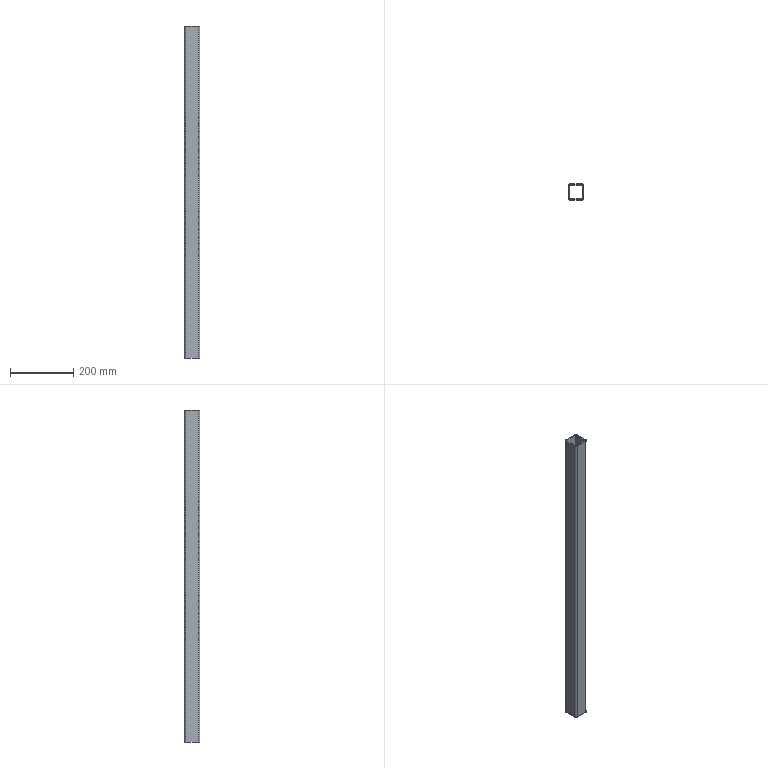Part | SolidWorks | 1 solid | 18 faces | box 50 x 50 x 1050 mm | volume 567864 mm3 | plane 10 | cylinder 8 | commonest cylinder face diameters 6 x4 12 x4
STEP:
#1=CARTESIAN_POINT('',(19.,25.,525.));
#2=VERTEX_POINT('',#1);
#3=CARTESIAN_POINT('',(25.,19.,525.));
#4=VERTEX_POINT('',#3);
#5=CARTESIAN_POINT('',(19.,19.,525.));
#6=DIRECTION('',(0.,0.,-1.));
#7=DIRECTION('',(-1.,0.,0.));
#8=AXIS2_PLACEMENT_3D('',#5,#6,#7);
#9=CIRCLE('',#8,6.);
#10=EDGE_CURVE('',#2,#4,#9,.T.);
#11=ORIENTED_EDGE('',*,*,#10,.T.);
#12=CARTESIAN_POINT('',(25.,19.,-525.));
#13=VERTEX_POINT('',#12);
#14=CARTESIAN_POINT('',(25.,19.,-525.));
#15=DIRECTION('',(0.,0.,1.));
#16=VECTOR('',#15,1000.);
#17=LINE('',#14,#16);
#18=EDGE_CURVE('',#13,#4,#17,.T.);
#19=ORIENTED_EDGE('',*,*,#18,.F.);
#20=CARTESIAN_POINT('',(19.,25.,-525.));
#21=VERTEX_POINT('',#20);
#22=CARTESIAN_POINT('',(19.,19.,-525.));
#23=DIRECTION('',(0.,0.,-1.));
#24=DIRECTION('',(-1.,0.,0.));
#25=AXIS2_PLACEMENT_3D('',#22,#23,#24);
#26=CIRCLE('',#25,6.);
#27=EDGE_CURVE('',#21,#13,#26,.T.);
#28=ORIENTED_EDGE('',*,*,#27,.F.);
#29=CARTESIAN_POINT('',(19.,25.,-525.));
#30=DIRECTION('',(0.,0.,1.));
#31=VECTOR('',#30,1000.);
#32=LINE('',#29,#31);
#33=EDGE_CURVE('',#21,#2,#32,.T.);
#34=ORIENTED_EDGE('',*,*,#33,.T.);
#35=EDGE_LOOP('',(#11,#19,#28,#34));
#36=FACE_OUTER_BOUND('',#35,.T.);
#37=CARTESIAN_POINT('',(19.,19.,-525.));
#38=DIRECTION('',(0.,0.,1.));
#39=DIRECTION('',(1.,0.,0.));
#40=AXIS2_PLACEMENT_3D('',#37,#38,#39);
#41=CYLINDRICAL_SURFACE('',#40,6.);
#42=ADVANCED_FACE('',(#36),#41,.T.);
#43=CARTESIAN_POINT('',(25.,-19.,525.));
#44=VERTEX_POINT('',#43);
#45=CARTESIAN_POINT('',(25.,19.,525.));
#46=DIRECTION('',(0.,-1.,0.));
#47=VECTOR('',#46,1000.);
#48=LINE('',#45,#47);
#49=EDGE_CURVE('',#4,#44,#48,.T.);
#50=ORIENTED_EDGE('',*,*,#49,.T.);
#51=CARTESIAN_POINT('',(25.,-19.,-525.));
#52=VERTEX_POINT('',#51);
#53=CARTESIAN_POINT('',(25.,-19.,-525.));
#54=DIRECTION('',(0.,0.,1.));
#55=VECTOR('',#54,1000.);
#56=LINE('',#53,#55);
#57=EDGE_CURVE('',#52,#44,#56,.T.);
#58=ORIENTED_EDGE('',*,*,#57,.F.);
#59=CARTESIAN_POINT('',(25.,19.,-525.));
#60=DIRECTION('',(0.,-1.,0.));
#61=VECTOR('',#60,1000.);
#62=LINE('',#59,#61);
#63=EDGE_CURVE('',#13,#52,#62,.T.);
#64=ORIENTED_EDGE('',*,*,#63,.F.);
#65=ORIENTED_EDGE('',*,*,#18,.T.);
#66=EDGE_LOOP('',(#50,#58,#64,#65));
#67=FACE_OUTER_BOUND('',#66,.T.);
#68=CARTESIAN_POINT('',(25.,19.,-525.));
#69=DIRECTION('',(-1.,0.,0.));
#70=DIRECTION('',(0.,0.,1.));
#71=AXIS2_PLACEMENT_3D('',#68,#69,#70);
#72=PLANE('',#71);
#73=ADVANCED_FACE('',(#67),#72,.F.);
#74=CARTESIAN_POINT('',(19.,-25.,525.));
#75=VERTEX_POINT('',#74);
#76=CARTESIAN_POINT('',(19.,-19.,525.));
#77=DIRECTION('',(0.,0.,-1.));
#78=DIRECTION('',(-1.,0.,0.));
#79=AXIS2_PLACEMENT_3D('',#76,#77,#78);
#80=CIRCLE('',#79,6.);
#81=EDGE_CURVE('',#44,#75,#80,.T.);
#82=ORIENTED_EDGE('',*,*,#81,.T.);
#83=CARTESIAN_POINT('',(19.,-25.,-525.));
#84=VERTEX_POINT('',#83);
#85=CARTESIAN_POINT('',(19.,-25.,-525.));
#86=DIRECTION('',(0.,0.,1.));
#87=VECTOR('',#86,1000.);
#88=LINE('',#85,#87);
#89=EDGE_CURVE('',#84,#75,#88,.T.);
#90=ORIENTED_EDGE('',*,*,#89,.F.);
#91=CARTESIAN_POINT('',(19.,-19.,-525.));
#92=DIRECTION('',(0.,0.,-1.));
#93=DIRECTION('',(-1.,0.,0.));
#94=AXIS2_PLACEMENT_3D('',#91,#92,#93);
#95=CIRCLE('',#94,6.);
#96=EDGE_CURVE('',#52,#84,#95,.T.);
#97=ORIENTED_EDGE('',*,*,#96,.F.);
#98=ORIENTED_EDGE('',*,*,#57,.T.);
#99=EDGE_LOOP('',(#82,#90,#97,#98));
#100=FACE_OUTER_BOUND('',#99,.T.);
#101=CARTESIAN_POINT('',(19.,-19.,-525.));
#102=DIRECTION('',(0.,0.,1.));
#103=DIRECTION('',(1.,0.,0.));
#104=AXIS2_PLACEMENT_3D('',#101,#102,#103);
#105=CYLINDRICAL_SURFACE('',#104,6.);
#106=ADVANCED_FACE('',(#100),#105,.T.);
#107=CARTESIAN_POINT('',(-19.,-25.,525.));
#108=VERTEX_POINT('',#107);
#109=CARTESIAN_POINT('',(-19.,-25.,525.));
#110=DIRECTION('',(-1.,0.,0.));
#111=VECTOR('',#110,1000.);
#112=LINE('',#109,#111);
#113=EDGE_CURVE('',#75,#108,#112,.T.);
#114=ORIENTED_EDGE('',*,*,#113,.T.);
#115=CARTESIAN_POINT('',(-19.,-25.,-525.));
#116=VERTEX_POINT('',#115);
#117=CARTESIAN_POINT('',(-19.,-25.,-525.));
#118=DIRECTION('',(0.,0.,1.));
#119=VECTOR('',#118,1000.);
#120=LINE('',#117,#119);
#121=EDGE_CURVE('',#116,#108,#120,.T.);
#122=ORIENTED_EDGE('',*,*,#121,.F.);
#123=CARTESIAN_POINT('',(-19.,-25.,-525.));
#124=DIRECTION('',(-1.,0.,0.));
#125=VECTOR('',#124,1000.);
#126=LINE('',#123,#125);
#127=EDGE_CURVE('',#84,#116,#126,.T.);
#128=ORIENTED_EDGE('',*,*,#127,.F.);
#129=ORIENTED_EDGE('',*,*,#89,.T.);
#130=EDGE_LOOP('',(#114,#122,#128,#129));
#131=FACE_OUTER_BOUND('',#130,.T.);
#132=CARTESIAN_POINT('',(-19.,-25.,-525.));
#133=DIRECTION('',(0.,1.,0.));
#134=DIRECTION('',(0.,0.,1.));
#135=AXIS2_PLACEMENT_3D('',#132,#133,#134);
#136=PLANE('',#135);
#137=ADVANCED_FACE('',(#131),#136,.F.);
#138=CARTESIAN_POINT('',(-25.,-19.,525.));
#139=VERTEX_POINT('',#138);
#140=CARTESIAN_POINT('',(-19.,-19.,525.));
#141=DIRECTION('',(0.,0.,-1.));
#142=DIRECTION('',(-1.,0.,0.));
#143=AXIS2_PLACEMENT_3D('',#140,#141,#142);
#144=CIRCLE('',#143,6.);
#145=EDGE_CURVE('',#108,#139,#144,.T.);
#146=ORIENTED_EDGE('',*,*,#145,.T.);
#147=CARTESIAN_POINT('',(-25.,-19.,-525.));
#148=VERTEX_POINT('',#147);
#149=CARTESIAN_POINT('',(-25.,-19.,-525.));
#150=DIRECTION('',(0.,0.,1.));
#151=VECTOR('',#150,1000.);
#152=LINE('',#149,#151);
#153=EDGE_CURVE('',#148,#139,#152,.T.);
#154=ORIENTED_EDGE('',*,*,#153,.F.);
#155=CARTESIAN_POINT('',(-19.,-19.,-525.));
#156=DIRECTION('',(0.,0.,-1.));
#157=DIRECTION('',(-1.,0.,0.));
#158=AXIS2_PLACEMENT_3D('',#155,#156,#157);
#159=CIRCLE('',#158,6.);
#160=EDGE_CURVE('',#116,#148,#159,.T.);
#161=ORIENTED_EDGE('',*,*,#160,.F.);
#162=ORIENTED_EDGE('',*,*,#121,.T.);
#163=EDGE_LOOP('',(#146,#154,#161,#162));
#164=FACE_OUTER_BOUND('',#163,.T.);
#165=CARTESIAN_POINT('',(-19.,-19.,-525.));
#166=DIRECTION('',(0.,0.,1.));
#167=DIRECTION('',(1.,0.,0.));
#168=AXIS2_PLACEMENT_3D('',#165,#166,#167);
#169=CYLINDRICAL_SURFACE('',#168,6.);
#170=ADVANCED_FACE('',(#164),#169,.T.);
#171=CARTESIAN_POINT('',(-25.,19.,525.));
#172=VERTEX_POINT('',#171);
#173=CARTESIAN_POINT('',(-25.,-19.,525.));
#174=DIRECTION('',(0.,1.,0.));
#175=VECTOR('',#174,1000.);
#176=LINE('',#173,#175);
#177=EDGE_CURVE('',#139,#172,#176,.T.);
#178=ORIENTED_EDGE('',*,*,#177,.T.);
#179=CARTESIAN_POINT('',(-25.,19.,-525.));
#180=VERTEX_POINT('',#179);
#181=CARTESIAN_POINT('',(-25.,19.,-525.));
#182=DIRECTION('',(0.,0.,1.));
#183=VECTOR('',#182,1000.);
#184=LINE('',#181,#183);
#185=EDGE_CURVE('',#180,#172,#184,.T.);
#186=ORIENTED_EDGE('',*,*,#185,.F.);
#187=CARTESIAN_POINT('',(-25.,-19.,-525.));
#188=DIRECTION('',(0.,1.,0.));
#189=VECTOR('',#188,1000.);
#190=LINE('',#187,#189);
#191=EDGE_CURVE('',#148,#180,#190,.T.);
#192=ORIENTED_EDGE('',*,*,#191,.F.);
#193=ORIENTED_EDGE('',*,*,#153,.T.);
#194=EDGE_LOOP('',(#178,#186,#192,#193));
#195=FACE_OUTER_BOUND('',#194,.T.);
#196=CARTESIAN_POINT('',(-25.,-19.,-525.));
#197=DIRECTION('',(1.,0.,0.));
#198=DIRECTION('',(0.,0.,-1.));
#199=AXIS2_PLACEMENT_3D('',#196,#197,#198);
#200=PLANE('',#199);
#201=ADVANCED_FACE('',(#195),#200,.F.);
#202=CARTESIAN_POINT('',(-19.,25.,525.));
#203=VERTEX_POINT('',#202);
#204=CARTESIAN_POINT('',(-19.,19.,525.));
#205=DIRECTION('',(0.,0.,-1.));
#206=DIRECTION('',(-1.,0.,0.));
#207=AXIS2_PLACEMENT_3D('',#204,#205,#206);
#208=CIRCLE('',#207,6.);
#209=EDGE_CURVE('',#172,#203,#208,.T.);
#210=ORIENTED_EDGE('',*,*,#209,.T.);
#211=CARTESIAN_POINT('',(-19.,25.,-525.));
#212=VERTEX_POINT('',#211);
#213=CARTESIAN_POINT('',(-19.,25.,-525.));
#214=DIRECTION('',(0.,0.,1.));
#215=VECTOR('',#214,1000.);
#216=LINE('',#213,#215);
#217=EDGE_CURVE('',#212,#203,#216,.T.);
#218=ORIENTED_EDGE('',*,*,#217,.F.);
#219=CARTESIAN_POINT('',(-19.,19.,-525.));
#220=DIRECTION('',(0.,0.,-1.));
#221=DIRECTION('',(-1.,0.,0.));
#222=AXIS2_PLACEMENT_3D('',#219,#220,#221);
#223=CIRCLE('',#222,6.);
#224=EDGE_CURVE('',#180,#212,#223,.T.);
#225=ORIENTED_EDGE('',*,*,#224,.F.);
#226=ORIENTED_EDGE('',*,*,#185,.T.);
#227=EDGE_LOOP('',(#210,#218,#225,#226));
#228=FACE_OUTER_BOUND('',#227,.T.);
#229=CARTESIAN_POINT('',(-19.,19.,-525.));
#230=DIRECTION('',(0.,0.,1.));
#231=DIRECTION('',(1.,0.,0.));
#232=AXIS2_PLACEMENT_3D('',#229,#230,#231);
#233=CYLINDRICAL_SURFACE('',#232,6.);
#234=ADVANCED_FACE('',(#228),#233,.T.);
#235=CARTESIAN_POINT('',(22.,-19.,525.));
#236=VERTEX_POINT('',#235);
#237=CARTESIAN_POINT('',(19.,-22.,525.));
#238=VERTEX_POINT('',#237);
#239=CARTESIAN_POINT('',(19.,-19.,525.));
#240=DIRECTION('',(0.,0.,-1.));
#241=DIRECTION('',(-1.,0.,0.));
#242=AXIS2_PLACEMENT_3D('',#239,#240,#241);
#243=CIRCLE('',#242,3.);
#244=EDGE_CURVE('',#236,#238,#243,.T.);
#245=ORIENTED_EDGE('',*,*,#244,.F.);
#246=CARTESIAN_POINT('',(22.,-19.,-525.));
#247=VERTEX_POINT('',#246);
#248=CARTESIAN_POINT('',(22.,-19.,-525.));
#249=DIRECTION('',(0.,0.,1.));
#250=VECTOR('',#249,1000.);
#251=LINE('',#248,#250);
#252=EDGE_CURVE('',#247,#236,#251,.T.);
#253=ORIENTED_EDGE('',*,*,#252,.F.);
#254=CARTESIAN_POINT('',(19.,-22.,-525.));
#255=VERTEX_POINT('',#254);
#256=CARTESIAN_POINT('',(19.,-19.,-525.));
#257=DIRECTION('',(0.,0.,-1.));
#258=DIRECTION('',(-1.,0.,0.));
#259=AXIS2_PLACEMENT_3D('',#256,#257,#258);
#260=CIRCLE('',#259,3.);
#261=EDGE_CURVE('',#247,#255,#260,.T.);
#262=ORIENTED_EDGE('',*,*,#261,.T.);
#263=CARTESIAN_POINT('',(19.,-22.,-525.));
#264=DIRECTION('',(0.,0.,1.));
#265=VECTOR('',#264,1000.);
#266=LINE('',#263,#265);
#267=EDGE_CURVE('',#255,#238,#266,.T.);
#268=ORIENTED_EDGE('',*,*,#267,.T.);
#269=EDGE_LOOP('',(#245,#253,#262,#268));
#270=FACE_OUTER_BOUND('',#269,.T.);
#271=CARTESIAN_POINT('',(19.,-19.,-525.));
#272=DIRECTION('',(0.,0.,1.));
#273=DIRECTION('',(1.,0.,0.));
#274=AXIS2_PLACEMENT_3D('',#271,#272,#273);
#275=CYLINDRICAL_SURFACE('',#274,3.);
#276=ADVANCED_FACE('',(#270),#275,.F.);
#277=CARTESIAN_POINT('',(22.,19.,525.));
#278=VERTEX_POINT('',#277);
#279=CARTESIAN_POINT('',(22.,19.,525.));
#280=DIRECTION('',(0.,-1.,0.));
#281=VECTOR('',#280,1000.);
#282=LINE('',#279,#281);
#283=EDGE_CURVE('',#278,#236,#282,.T.);
#284=ORIENTED_EDGE('',*,*,#283,.F.);
#285=CARTESIAN_POINT('',(22.,19.,-525.));
#286=VERTEX_POINT('',#285);
#287=CARTESIAN_POINT('',(22.,19.,-525.));
#288=DIRECTION('',(0.,0.,1.));
#289=VECTOR('',#288,1000.);
#290=LINE('',#287,#289);
#291=EDGE_CURVE('',#286,#278,#290,.T.);
#292=ORIENTED_EDGE('',*,*,#291,.F.);
#293=CARTESIAN_POINT('',(22.,19.,-525.));
#294=DIRECTION('',(0.,-1.,0.));
#295=VECTOR('',#294,1000.);
#296=LINE('',#293,#295);
#297=EDGE_CURVE('',#286,#247,#296,.T.);
#298=ORIENTED_EDGE('',*,*,#297,.T.);
#299=ORIENTED_EDGE('',*,*,#252,.T.);
#300=EDGE_LOOP('',(#284,#292,#298,#299));
#301=FACE_OUTER_BOUND('',#300,.T.);
#302=CARTESIAN_POINT('',(22.,19.,-525.));
#303=DIRECTION('',(-1.,0.,0.));
#304=DIRECTION('',(0.,0.,1.));
#305=AXIS2_PLACEMENT_3D('',#302,#303,#304);
#306=PLANE('',#305);
#307=ADVANCED_FACE('',(#301),#306,.T.);
#308=CARTESIAN_POINT('',(19.,22.,525.));
#309=VERTEX_POINT('',#308);
#310=CARTESIAN_POINT('',(19.,19.,525.));
#311=DIRECTION('',(0.,0.,-1.));
#312=DIRECTION('',(-1.,0.,0.));
#313=AXIS2_PLACEMENT_3D('',#310,#311,#312);
#314=CIRCLE('',#313,3.);
#315=EDGE_CURVE('',#309,#278,#314,.T.);
#316=ORIENTED_EDGE('',*,*,#315,.F.);
#317=CARTESIAN_POINT('',(19.,22.,-525.));
#318=VERTEX_POINT('',#317);
#319=CARTESIAN_POINT('',(19.,22.,-525.));
#320=DIRECTION('',(0.,0.,1.));
#321=VECTOR('',#320,1000.);
#322=LINE('',#319,#321);
#323=EDGE_CURVE('',#318,#309,#322,.T.);
#324=ORIENTED_EDGE('',*,*,#323,.F.);
#325=CARTESIAN_POINT('',(19.,19.,-525.));
#326=DIRECTION('',(0.,0.,-1.));
#327=DIRECTION('',(-1.,0.,0.));
#328=AXIS2_PLACEMENT_3D('',#325,#326,#327);
#329=CIRCLE('',#328,3.);
#330=EDGE_CURVE('',#318,#286,#329,.T.);
#331=ORIENTED_EDGE('',*,*,#330,.T.);
#332=ORIENTED_EDGE('',*,*,#291,.T.);
#333=EDGE_LOOP('',(#316,#324,#331,#332));
#334=FACE_OUTER_BOUND('',#333,.T.);
#335=CARTESIAN_POINT('',(19.,19.,-525.));
#336=DIRECTION('',(0.,0.,1.));
#337=DIRECTION('',(1.,0.,0.));
#338=AXIS2_PLACEMENT_3D('',#335,#336,#337);
#339=CYLINDRICAL_SURFACE('',#338,3.);
#340=ADVANCED_FACE('',(#334),#339,.F.);
#341=CARTESIAN_POINT('',(-19.,22.,525.));
#342=VERTEX_POINT('',#341);
#343=CARTESIAN_POINT('',(19.,22.,525.));
#344=DIRECTION('',(1.,0.,0.));
#345=VECTOR('',#344,1000.);
#346=LINE('',#343,#345);
#347=EDGE_CURVE('',#342,#309,#346,.T.);
#348=ORIENTED_EDGE('',*,*,#347,.F.);
#349=CARTESIAN_POINT('',(-19.,22.,-525.));
#350=VERTEX_POINT('',#349);
#351=CARTESIAN_POINT('',(-19.,22.,-525.));
#352=DIRECTION('',(0.,0.,1.));
#353=VECTOR('',#352,1000.);
#354=LINE('',#351,#353);
#355=EDGE_CURVE('',#350,#342,#354,.T.);
#356=ORIENTED_EDGE('',*,*,#355,.F.);
#357=CARTESIAN_POINT('',(19.,22.,-525.));
#358=DIRECTION('',(1.,0.,0.));
#359=VECTOR('',#358,1000.);
#360=LINE('',#357,#359);
#361=EDGE_CURVE('',#350,#318,#360,.T.);
#362=ORIENTED_EDGE('',*,*,#361,.T.);
#363=ORIENTED_EDGE('',*,*,#323,.T.);
#364=EDGE_LOOP('',(#348,#356,#362,#363));
#365=FACE_OUTER_BOUND('',#364,.T.);
#366=CARTESIAN_POINT('',(19.,22.,-525.));
#367=DIRECTION('',(0.,-1.,0.));
#368=DIRECTION('',(0.,0.,-1.));
#369=AXIS2_PLACEMENT_3D('',#366,#367,#368);
#370=PLANE('',#369);
#371=ADVANCED_FACE('',(#365),#370,.T.);
#372=CARTESIAN_POINT('',(-22.,19.,525.));
#373=VERTEX_POINT('',#372);
#374=CARTESIAN_POINT('',(-19.,19.,525.));
#375=DIRECTION('',(0.,0.,-1.));
#376=DIRECTION('',(-1.,0.,0.));
#377=AXIS2_PLACEMENT_3D('',#374,#375,#376);
#378=CIRCLE('',#377,3.);
#379=EDGE_CURVE('',#373,#342,#378,.T.);
#380=ORIENTED_EDGE('',*,*,#379,.F.);
#381=CARTESIAN_POINT('',(-22.,19.,-525.));
#382=VERTEX_POINT('',#381);
#383=CARTESIAN_POINT('',(-22.,19.,-525.));
#384=DIRECTION('',(0.,0.,1.));
#385=VECTOR('',#384,1000.);
#386=LINE('',#383,#385);
#387=EDGE_CURVE('',#382,#373,#386,.T.);
#388=ORIENTED_EDGE('',*,*,#387,.F.);
#389=CARTESIAN_POINT('',(-19.,19.,-525.));
#390=DIRECTION('',(0.,0.,-1.));
#391=DIRECTION('',(-1.,0.,0.));
#392=AXIS2_PLACEMENT_3D('',#389,#390,#391);
#393=CIRCLE('',#392,3.);
#394=EDGE_CURVE('',#382,#350,#393,.T.);
#395=ORIENTED_EDGE('',*,*,#394,.T.);
#396=ORIENTED_EDGE('',*,*,#355,.T.);
#397=EDGE_LOOP('',(#380,#388,#395,#396));
#398=FACE_OUTER_BOUND('',#397,.T.);
#399=CARTESIAN_POINT('',(-19.,19.,-525.));
#400=DIRECTION('',(0.,0.,1.));
#401=DIRECTION('',(1.,0.,0.));
#402=AXIS2_PLACEMENT_3D('',#399,#400,#401);
#403=CYLINDRICAL_SURFACE('',#402,3.);
#404=ADVANCED_FACE('',(#398),#403,.F.);
#405=CARTESIAN_POINT('',(-22.,-19.,525.));
#406=VERTEX_POINT('',#405);
#407=CARTESIAN_POINT('',(-22.,-19.,525.));
#408=DIRECTION('',(0.,1.,0.));
#409=VECTOR('',#408,1000.);
#410=LINE('',#407,#409);
#411=EDGE_CURVE('',#406,#373,#410,.T.);
#412=ORIENTED_EDGE('',*,*,#411,.F.);
#413=CARTESIAN_POINT('',(-22.,-19.,-525.));
#414=VERTEX_POINT('',#413);
#415=CARTESIAN_POINT('',(-22.,-19.,-525.));
#416=DIRECTION('',(0.,0.,1.));
#417=VECTOR('',#416,1000.);
#418=LINE('',#415,#417);
#419=EDGE_CURVE('',#414,#406,#418,.T.);
#420=ORIENTED_EDGE('',*,*,#419,.F.);
#421=CARTESIAN_POINT('',(-22.,-19.,-525.));
#422=DIRECTION('',(0.,1.,0.));
#423=VECTOR('',#422,1000.);
#424=LINE('',#421,#423);
#425=EDGE_CURVE('',#414,#382,#424,.T.);
#426=ORIENTED_EDGE('',*,*,#425,.T.);
#427=ORIENTED_EDGE('',*,*,#387,.T.);
#428=EDGE_LOOP('',(#412,#420,#426,#427));
#429=FACE_OUTER_BOUND('',#428,.T.);
#430=CARTESIAN_POINT('',(-22.,-19.,-525.));
#431=DIRECTION('',(1.,0.,0.));
#432=DIRECTION('',(0.,0.,-1.));
#433=AXIS2_PLACEMENT_3D('',#430,#431,#432);
#434=PLANE('',#433);
#435=ADVANCED_FACE('',(#429),#434,.T.);
#436=CARTESIAN_POINT('',(-19.,-22.,525.));
#437=VERTEX_POINT('',#436);
#438=CARTESIAN_POINT('',(-19.,-19.,525.));
#439=DIRECTION('',(0.,0.,-1.));
#440=DIRECTION('',(-1.,0.,0.));
#441=AXIS2_PLACEMENT_3D('',#438,#439,#440);
#442=CIRCLE('',#441,3.);
#443=EDGE_CURVE('',#437,#406,#442,.T.);
#444=ORIENTED_EDGE('',*,*,#443,.F.);
#445=CARTESIAN_POINT('',(-19.,-22.,-525.));
#446=VERTEX_POINT('',#445);
#447=CARTESIAN_POINT('',(-19.,-22.,-525.));
#448=DIRECTION('',(0.,0.,1.));
#449=VECTOR('',#448,1000.);
#450=LINE('',#447,#449);
#451=EDGE_CURVE('',#446,#437,#450,.T.);
#452=ORIENTED_EDGE('',*,*,#451,.F.);
#453=CARTESIAN_POINT('',(-19.,-19.,-525.));
#454=DIRECTION('',(0.,0.,-1.));
#455=DIRECTION('',(-1.,0.,0.));
#456=AXIS2_PLACEMENT_3D('',#453,#454,#455);
#457=CIRCLE('',#456,3.);
#458=EDGE_CURVE('',#446,#414,#457,.T.);
#459=ORIENTED_EDGE('',*,*,#458,.T.);
#460=ORIENTED_EDGE('',*,*,#419,.T.);
#461=EDGE_LOOP('',(#444,#452,#459,#460));
#462=FACE_OUTER_BOUND('',#461,.T.);
#463=CARTESIAN_POINT('',(-19.,-19.,-525.));
#464=DIRECTION('',(0.,0.,1.));
#465=DIRECTION('',(1.,0.,0.));
#466=AXIS2_PLACEMENT_3D('',#463,#464,#465);
#467=CYLINDRICAL_SURFACE('',#466,3.);
#468=ADVANCED_FACE('',(#462),#467,.F.);
#469=CARTESIAN_POINT('',(-19.,-22.,525.));
#470=DIRECTION('',(-1.,0.,0.));
#471=VECTOR('',#470,1000.);
#472=LINE('',#469,#471);
#473=EDGE_CURVE('',#238,#437,#472,.T.);
#474=ORIENTED_EDGE('',*,*,#473,.F.);
#475=ORIENTED_EDGE('',*,*,#267,.F.);
#476=CARTESIAN_POINT('',(-19.,-22.,-525.));
#477=DIRECTION('',(-1.,0.,0.));
#478=VECTOR('',#477,1000.);
#479=LINE('',#476,#478);
#480=EDGE_CURVE('',#255,#446,#479,.T.);
#481=ORIENTED_EDGE('',*,*,#480,.T.);
#482=ORIENTED_EDGE('',*,*,#451,.T.);
#483=EDGE_LOOP('',(#474,#475,#481,#482));
#484=FACE_OUTER_BOUND('',#483,.T.);
#485=CARTESIAN_POINT('',(-19.,-22.,-525.));
#486=DIRECTION('',(0.,1.,0.));
#487=DIRECTION('',(0.,0.,1.));
#488=AXIS2_PLACEMENT_3D('',#485,#486,#487);
#489=PLANE('',#488);
#490=ADVANCED_FACE('',(#484),#489,.T.);
#491=CARTESIAN_POINT('',(19.,25.,525.));
#492=DIRECTION('',(1.,0.,0.));
#493=VECTOR('',#492,1000.);
#494=LINE('',#491,#493);
#495=EDGE_CURVE('',#203,#2,#494,.T.);
#496=ORIENTED_EDGE('',*,*,#495,.T.);
#497=ORIENTED_EDGE('',*,*,#33,.F.);
#498=CARTESIAN_POINT('',(19.,25.,-525.));
#499=DIRECTION('',(1.,0.,0.));
#500=VECTOR('',#499,1000.);
#501=LINE('',#498,#500);
#502=EDGE_CURVE('',#212,#21,#501,.T.);
#503=ORIENTED_EDGE('',*,*,#502,.F.);
#504=ORIENTED_EDGE('',*,*,#217,.T.);
#505=EDGE_LOOP('',(#496,#497,#503,#504));
#506=FACE_OUTER_BOUND('',#505,.T.);
#507=CARTESIAN_POINT('',(19.,25.,-525.));
#508=DIRECTION('',(0.,-1.,0.));
#509=DIRECTION('',(0.,0.,-1.));
#510=AXIS2_PLACEMENT_3D('',#507,#508,#509);
#511=PLANE('',#510);
#512=ADVANCED_FACE('',(#506),#511,.F.);
#513=ORIENTED_EDGE('',*,*,#261,.F.);
#514=ORIENTED_EDGE('',*,*,#297,.F.);
#515=ORIENTED_EDGE('',*,*,#330,.F.);
#516=ORIENTED_EDGE('',*,*,#361,.F.);
#517=ORIENTED_EDGE('',*,*,#394,.F.);
#518=ORIENTED_EDGE('',*,*,#425,.F.);
#519=ORIENTED_EDGE('',*,*,#458,.F.);
#520=ORIENTED_EDGE('',*,*,#480,.F.);
#521=EDGE_LOOP('',(#513,#514,#515,#516,#517,#518,#519,#520));
#522=FACE_BOUND('',#521,.T.);
#523=ORIENTED_EDGE('',*,*,#27,.T.);
#524=ORIENTED_EDGE('',*,*,#63,.T.);
#525=ORIENTED_EDGE('',*,*,#96,.T.);
#526=ORIENTED_EDGE('',*,*,#127,.T.);
#527=ORIENTED_EDGE('',*,*,#160,.T.);
#528=ORIENTED_EDGE('',*,*,#191,.T.);
#529=ORIENTED_EDGE('',*,*,#224,.T.);
#530=ORIENTED_EDGE('',*,*,#502,.T.);
#531=EDGE_LOOP('',(#523,#524,#525,#526,#527,#528,#529,#530));
#532=FACE_OUTER_BOUND('',#531,.T.);
#533=CARTESIAN_POINT('',(19.,19.,-525.));
#534=DIRECTION('',(0.,0.,-1.));
#535=DIRECTION('',(-1.,0.,0.));
#536=AXIS2_PLACEMENT_3D('',#533,#534,#535);
#537=PLANE('',#536);
#538=ADVANCED_FACE('',(#522,#532),#537,.T.);
#539=ORIENTED_EDGE('',*,*,#244,.T.);
#540=ORIENTED_EDGE('',*,*,#473,.T.);
#541=ORIENTED_EDGE('',*,*,#443,.T.);
#542=ORIENTED_EDGE('',*,*,#411,.T.);
#543=ORIENTED_EDGE('',*,*,#379,.T.);
#544=ORIENTED_EDGE('',*,*,#347,.T.);
#545=ORIENTED_EDGE('',*,*,#315,.T.);
#546=ORIENTED_EDGE('',*,*,#283,.T.);
#547=EDGE_LOOP('',(#539,#540,#541,#542,#543,#544,#545,#546));
#548=FACE_BOUND('',#547,.T.);
#549=ORIENTED_EDGE('',*,*,#10,.F.);
#550=ORIENTED_EDGE('',*,*,#495,.F.);
#551=ORIENTED_EDGE('',*,*,#209,.F.);
#552=ORIENTED_EDGE('',*,*,#177,.F.);
#553=ORIENTED_EDGE('',*,*,#145,.F.);
#554=ORIENTED_EDGE('',*,*,#113,.F.);
#555=ORIENTED_EDGE('',*,*,#81,.F.);
#556=ORIENTED_EDGE('',*,*,#49,.F.);
#557=EDGE_LOOP('',(#549,#550,#551,#552,#553,#554,#555,#556));
#558=FACE_OUTER_BOUND('',#557,.T.);
#559=CARTESIAN_POINT('',(19.,19.,525.));
#560=DIRECTION('',(0.,0.,-1.));
#561=DIRECTION('',(-1.,0.,0.));
#562=AXIS2_PLACEMENT_3D('',#559,#560,#561);
#563=PLANE('',#562);
#564=ADVANCED_FACE('',(#548,#558),#563,.F.);
#565=CLOSED_SHELL('',(#42,#73,#106,#137,#170,#201,#234,#276,#307,#340,#371,#404,#435,#468,#490,#512,#538,#564));
#566=MANIFOLD_SOLID_BREP('',#565);
#567=CARTESIAN_POINT('',(0.,0.,0.));
#568=DIRECTION('',(0.,0.,1.));
#569=DIRECTION('',(1.,0.,0.));
#570=AXIS2_PLACEMENT_3D('',#567,#568,#569);
#571=(LENGTH_UNIT()NAMED_UNIT(*)SI_UNIT(.MILLI.,.METRE.));
#572=UNCERTAINTY_MEASURE_WITH_UNIT(LENGTH_MEASURE(0.00001),#571,'','');
#573=(NAMED_UNIT(*)PLANE_ANGLE_UNIT()SI_UNIT($,.RADIAN.));
#574=(NAMED_UNIT(*)SI_UNIT($,.STERADIAN.)SOLID_ANGLE_UNIT());
#575=(GEOMETRIC_REPRESENTATION_CONTEXT(3)GLOBAL_UNCERTAINTY_ASSIGNED_CONTEXT((#572))GLOBAL_UNIT_ASSIGNED_CONTEXT((#571,#573,#574))REPRESENTATION_CONTEXT('',''));
#576=ADVANCED_BREP_SHAPE_REPRESENTATION('',(#566,#570),#575);